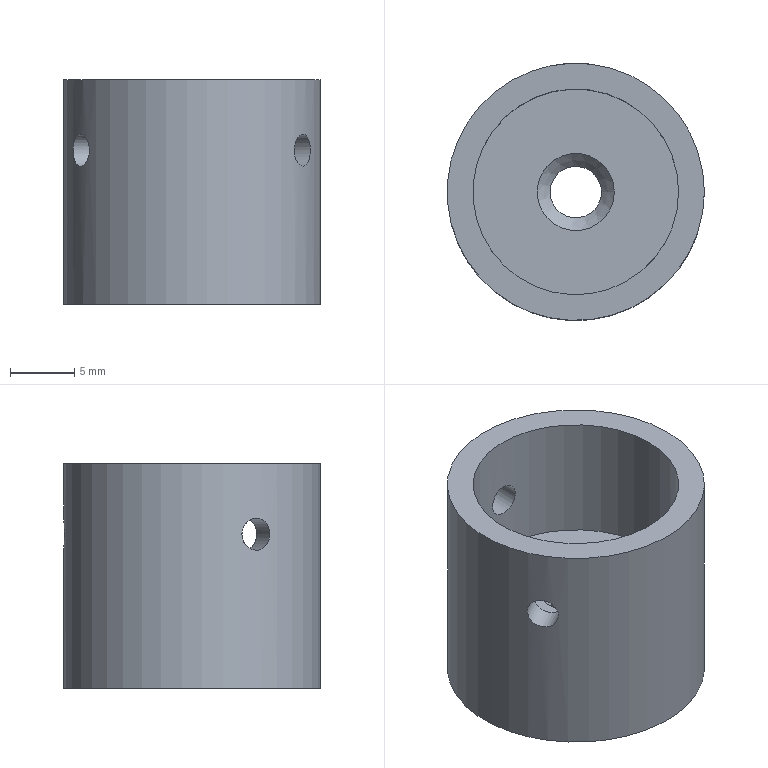Part | NX | features BREP 1, DATUM_CSYS 1 | 1 solid | 19 faces | box 20 x 20 x 17.5 mm | volume 3306 mm3 | cylinder 10 | plane 8 | cone 1 | commonest cylinder face diameters 6 x4 2.5 x3 4 x1 16 x1 20 x1
STEP:
#1=CARTESIAN_POINT('',(0.5952,-2.94,5.));
#2=VERTEX_POINT('',#1);
#3=CARTESIAN_POINT('',(2.94,-0.5952,5.));
#4=VERTEX_POINT('',#3);
#5=CARTESIAN_POINT('',(0.5952,-2.94,5.));
#6=DIRECTION('',(0.7071,0.7071,0.));
#7=VECTOR('',#6,1000.);
#8=LINE('',#5,#7);
#9=EDGE_CURVE('',#2,#4,#8,.T.);
#10=ORIENTED_EDGE('',*,*,#9,.F.);
#11=CARTESIAN_POINT('',(-0.5952,-2.94,5.));
#12=VERTEX_POINT('',#11);
#13=CARTESIAN_POINT('',(0.,0.,5.));
#14=DIRECTION('',(0.,0.,1.));
#15=DIRECTION('',(-0.1984,-0.9801,0.));
#16=AXIS2_PLACEMENT_3D('',#13,#14,#15);
#17=CIRCLE('',#16,3.);
#18=EDGE_CURVE('',#12,#2,#17,.T.);
#19=ORIENTED_EDGE('',*,*,#18,.F.);
#20=CARTESIAN_POINT('',(-2.94,-0.5952,5.));
#21=VERTEX_POINT('',#20);
#22=CARTESIAN_POINT('',(-2.94,-0.5952,5.));
#23=DIRECTION('',(0.7071,-0.7071,0.));
#24=VECTOR('',#23,1000.);
#25=LINE('',#22,#24);
#26=EDGE_CURVE('',#21,#12,#25,.T.);
#27=ORIENTED_EDGE('',*,*,#26,.F.);
#28=CARTESIAN_POINT('',(-2.94,0.5952,5.));
#29=VERTEX_POINT('',#28);
#30=CARTESIAN_POINT('',(0.,0.,5.));
#31=DIRECTION('',(0.,0.,1.));
#32=DIRECTION('',(-0.9801,0.1984,0.));
#33=AXIS2_PLACEMENT_3D('',#30,#31,#32);
#34=CIRCLE('',#33,3.);
#35=EDGE_CURVE('',#29,#21,#34,.T.);
#36=ORIENTED_EDGE('',*,*,#35,.F.);
#37=CARTESIAN_POINT('',(-0.5952,2.94,5.));
#38=VERTEX_POINT('',#37);
#39=CARTESIAN_POINT('',(-0.5952,2.94,5.));
#40=DIRECTION('',(-0.7071,-0.7071,0.));
#41=VECTOR('',#40,1000.);
#42=LINE('',#39,#41);
#43=EDGE_CURVE('',#38,#29,#42,.T.);
#44=ORIENTED_EDGE('',*,*,#43,.F.);
#45=CARTESIAN_POINT('',(0.5952,2.94,5.));
#46=VERTEX_POINT('',#45);
#47=CARTESIAN_POINT('',(0.,0.,5.));
#48=DIRECTION('',(0.,0.,1.));
#49=DIRECTION('',(0.1984,0.9801,0.));
#50=AXIS2_PLACEMENT_3D('',#47,#48,#49);
#51=CIRCLE('',#50,3.);
#52=EDGE_CURVE('',#46,#38,#51,.T.);
#53=ORIENTED_EDGE('',*,*,#52,.F.);
#54=CARTESIAN_POINT('',(2.94,0.5952,5.));
#55=VERTEX_POINT('',#54);
#56=CARTESIAN_POINT('',(2.94,0.5952,5.));
#57=DIRECTION('',(-0.7071,0.7071,0.));
#58=VECTOR('',#57,1000.);
#59=LINE('',#56,#58);
#60=EDGE_CURVE('',#55,#46,#59,.T.);
#61=ORIENTED_EDGE('',*,*,#60,.F.);
#62=CARTESIAN_POINT('',(0.,0.,5.));
#63=DIRECTION('',(0.,0.,1.));
#64=DIRECTION('',(0.9801,-0.1984,0.));
#65=AXIS2_PLACEMENT_3D('',#62,#63,#64);
#66=CIRCLE('',#65,3.);
#67=EDGE_CURVE('',#4,#55,#66,.T.);
#68=ORIENTED_EDGE('',*,*,#67,.F.);
#69=EDGE_LOOP('',(#10,#19,#27,#36,#44,#53,#61,#68));
#70=FACE_BOUND('',#69,.T.);
#71=CARTESIAN_POINT('',(2.,0.,5.));
#72=VERTEX_POINT('',#71);
#73=CARTESIAN_POINT('',(0.,0.,5.));
#74=DIRECTION('',(0.,0.,-1.));
#75=DIRECTION('',(1.,0.,0.));
#76=AXIS2_PLACEMENT_3D('',#73,#74,#75);
#77=CIRCLE('',#76,2.);
#78=EDGE_CURVE('',#72,#72,#77,.T.);
#79=ORIENTED_EDGE('',*,*,#78,.F.);
#80=EDGE_LOOP('',(#79));
#81=FACE_BOUND('',#80,.T.);
#82=CARTESIAN_POINT('',(0.,0.,5.));
#83=DIRECTION('',(0.,0.,1.));
#84=DIRECTION('',(1.,0.,0.));
#85=AXIS2_PLACEMENT_3D('',#82,#83,#84);
#86=PLANE('',#85);
#87=ADVANCED_FACE('',(#70,#81),#86,.F.);
#88=ORIENTED_EDGE('',*,*,#67,.T.);
#89=CARTESIAN_POINT('',(2.94,0.5952,0.5));
#90=VERTEX_POINT('',#89);
#91=CARTESIAN_POINT('',(2.94,0.5952,5.));
#92=DIRECTION('',(0.,0.,-1.));
#93=VECTOR('',#92,1000.);
#94=LINE('',#91,#93);
#95=EDGE_CURVE('',#55,#90,#94,.T.);
#96=ORIENTED_EDGE('',*,*,#95,.T.);
#97=CARTESIAN_POINT('',(2.94,-0.5952,0.5));
#98=VERTEX_POINT('',#97);
#99=CARTESIAN_POINT('',(0.,0.,0.5));
#100=DIRECTION('',(0.,0.,-1.));
#101=DIRECTION('',(0.9801,0.1984,0.));
#102=AXIS2_PLACEMENT_3D('',#99,#100,#101);
#103=CIRCLE('',#102,3.);
#104=EDGE_CURVE('',#90,#98,#103,.T.);
#105=ORIENTED_EDGE('',*,*,#104,.T.);
#106=CARTESIAN_POINT('',(2.94,-0.5952,5.));
#107=DIRECTION('',(0.,0.,-1.));
#108=VECTOR('',#107,1000.);
#109=LINE('',#106,#108);
#110=EDGE_CURVE('',#4,#98,#109,.T.);
#111=ORIENTED_EDGE('',*,*,#110,.F.);
#112=EDGE_LOOP('',(#88,#96,#105,#111));
#113=FACE_BOUND('',#112,.T.);
#114=CARTESIAN_POINT('',(0.,0.,5.));
#115=DIRECTION('',(0.,0.,-1.));
#116=DIRECTION('',(-0.9801,0.1984,0.));
#117=AXIS2_PLACEMENT_3D('',#114,#115,#116);
#118=CYLINDRICAL_SURFACE('',#117,3.);
#119=ADVANCED_FACE('',(#113),#118,.F.);
#120=ORIENTED_EDGE('',*,*,#60,.T.);
#121=CARTESIAN_POINT('',(0.5952,2.94,0.5));
#122=VERTEX_POINT('',#121);
#123=CARTESIAN_POINT('',(0.5952,2.94,5.));
#124=DIRECTION('',(0.,0.,-1.));
#125=VECTOR('',#124,1000.);
#126=LINE('',#123,#125);
#127=EDGE_CURVE('',#46,#122,#126,.T.);
#128=ORIENTED_EDGE('',*,*,#127,.T.);
#129=CARTESIAN_POINT('',(0.5952,2.94,0.5));
#130=DIRECTION('',(0.7071,-0.7071,0.));
#131=VECTOR('',#130,1000.);
#132=LINE('',#129,#131);
#133=EDGE_CURVE('',#122,#90,#132,.T.);
#134=ORIENTED_EDGE('',*,*,#133,.T.);
#135=ORIENTED_EDGE('',*,*,#95,.F.);
#136=EDGE_LOOP('',(#120,#128,#134,#135));
#137=FACE_BOUND('',#136,.T.);
#138=CARTESIAN_POINT('',(1.768,1.768,1.85));
#139=DIRECTION('',(-0.7071,-0.7071,0.));
#140=DIRECTION('',(0.7071,-0.7071,0.));
#141=AXIS2_PLACEMENT_3D('',#138,#139,#140);
#142=PLANE('',#141);
#143=ADVANCED_FACE('',(#137),#142,.T.);
#144=ORIENTED_EDGE('',*,*,#52,.T.);
#145=CARTESIAN_POINT('',(-0.5952,2.94,0.5));
#146=VERTEX_POINT('',#145);
#147=CARTESIAN_POINT('',(-0.5952,2.94,5.));
#148=DIRECTION('',(0.,0.,-1.));
#149=VECTOR('',#148,1000.);
#150=LINE('',#147,#149);
#151=EDGE_CURVE('',#38,#146,#150,.T.);
#152=ORIENTED_EDGE('',*,*,#151,.T.);
#153=CARTESIAN_POINT('',(0.,0.,0.5));
#154=DIRECTION('',(0.,0.,-1.));
#155=DIRECTION('',(-0.1984,0.9801,0.));
#156=AXIS2_PLACEMENT_3D('',#153,#154,#155);
#157=CIRCLE('',#156,3.);
#158=EDGE_CURVE('',#146,#122,#157,.T.);
#159=ORIENTED_EDGE('',*,*,#158,.T.);
#160=ORIENTED_EDGE('',*,*,#127,.F.);
#161=EDGE_LOOP('',(#144,#152,#159,#160));
#162=FACE_BOUND('',#161,.T.);
#163=CARTESIAN_POINT('',(0.,0.,5.));
#164=DIRECTION('',(0.,0.,-1.));
#165=DIRECTION('',(-0.1984,-0.9801,0.));
#166=AXIS2_PLACEMENT_3D('',#163,#164,#165);
#167=CYLINDRICAL_SURFACE('',#166,3.);
#168=ADVANCED_FACE('',(#162),#167,.F.);
#169=ORIENTED_EDGE('',*,*,#43,.T.);
#170=CARTESIAN_POINT('',(-2.94,0.5952,0.5));
#171=VERTEX_POINT('',#170);
#172=CARTESIAN_POINT('',(-2.94,0.5952,5.));
#173=DIRECTION('',(0.,0.,-1.));
#174=VECTOR('',#173,1000.);
#175=LINE('',#172,#174);
#176=EDGE_CURVE('',#29,#171,#175,.T.);
#177=ORIENTED_EDGE('',*,*,#176,.T.);
#178=CARTESIAN_POINT('',(-2.94,0.5952,0.5));
#179=DIRECTION('',(0.7071,0.7071,0.));
#180=VECTOR('',#179,1000.);
#181=LINE('',#178,#180);
#182=EDGE_CURVE('',#171,#146,#181,.T.);
#183=ORIENTED_EDGE('',*,*,#182,.T.);
#184=ORIENTED_EDGE('',*,*,#151,.F.);
#185=EDGE_LOOP('',(#169,#177,#183,#184));
#186=FACE_BOUND('',#185,.T.);
#187=CARTESIAN_POINT('',(-1.768,1.768,1.85));
#188=DIRECTION('',(0.7071,-0.7071,0.));
#189=DIRECTION('',(0.7071,0.7071,0.));
#190=AXIS2_PLACEMENT_3D('',#187,#188,#189);
#191=PLANE('',#190);
#192=ADVANCED_FACE('',(#186),#191,.T.);
#193=ORIENTED_EDGE('',*,*,#35,.T.);
#194=CARTESIAN_POINT('',(-2.94,-0.5952,0.5));
#195=VERTEX_POINT('',#194);
#196=CARTESIAN_POINT('',(-2.94,-0.5952,5.));
#197=DIRECTION('',(0.,0.,-1.));
#198=VECTOR('',#197,1000.);
#199=LINE('',#196,#198);
#200=EDGE_CURVE('',#21,#195,#199,.T.);
#201=ORIENTED_EDGE('',*,*,#200,.T.);
#202=CARTESIAN_POINT('',(0.,0.,0.5));
#203=DIRECTION('',(0.,0.,-1.));
#204=DIRECTION('',(-0.9801,-0.1984,0.));
#205=AXIS2_PLACEMENT_3D('',#202,#203,#204);
#206=CIRCLE('',#205,3.);
#207=EDGE_CURVE('',#195,#171,#206,.T.);
#208=ORIENTED_EDGE('',*,*,#207,.T.);
#209=ORIENTED_EDGE('',*,*,#176,.F.);
#210=EDGE_LOOP('',(#193,#201,#208,#209));
#211=FACE_BOUND('',#210,.T.);
#212=CARTESIAN_POINT('',(0.,0.,5.));
#213=DIRECTION('',(0.,0.,-1.));
#214=DIRECTION('',(0.9801,-0.1984,0.));
#215=AXIS2_PLACEMENT_3D('',#212,#213,#214);
#216=CYLINDRICAL_SURFACE('',#215,3.);
#217=ADVANCED_FACE('',(#211),#216,.F.);
#218=ORIENTED_EDGE('',*,*,#26,.T.);
#219=CARTESIAN_POINT('',(-0.5952,-2.94,0.5));
#220=VERTEX_POINT('',#219);
#221=CARTESIAN_POINT('',(-0.5952,-2.94,5.));
#222=DIRECTION('',(0.,0.,-1.));
#223=VECTOR('',#222,1000.);
#224=LINE('',#221,#223);
#225=EDGE_CURVE('',#12,#220,#224,.T.);
#226=ORIENTED_EDGE('',*,*,#225,.T.);
#227=CARTESIAN_POINT('',(-0.5952,-2.94,0.5));
#228=DIRECTION('',(-0.7071,0.7071,0.));
#229=VECTOR('',#228,1000.);
#230=LINE('',#227,#229);
#231=EDGE_CURVE('',#220,#195,#230,.T.);
#232=ORIENTED_EDGE('',*,*,#231,.T.);
#233=ORIENTED_EDGE('',*,*,#200,.F.);
#234=EDGE_LOOP('',(#218,#226,#232,#233));
#235=FACE_BOUND('',#234,.T.);
#236=CARTESIAN_POINT('',(-1.768,-1.768,1.85));
#237=DIRECTION('',(0.7071,0.7071,0.));
#238=DIRECTION('',(-0.7071,0.7071,0.));
#239=AXIS2_PLACEMENT_3D('',#236,#237,#238);
#240=PLANE('',#239);
#241=ADVANCED_FACE('',(#235),#240,.T.);
#242=ORIENTED_EDGE('',*,*,#18,.T.);
#243=CARTESIAN_POINT('',(0.5952,-2.94,0.5));
#244=VERTEX_POINT('',#243);
#245=CARTESIAN_POINT('',(0.5952,-2.94,5.));
#246=DIRECTION('',(0.,0.,-1.));
#247=VECTOR('',#246,1000.);
#248=LINE('',#245,#247);
#249=EDGE_CURVE('',#2,#244,#248,.T.);
#250=ORIENTED_EDGE('',*,*,#249,.T.);
#251=CARTESIAN_POINT('',(0.,0.,0.5));
#252=DIRECTION('',(0.,0.,-1.));
#253=DIRECTION('',(0.1984,-0.9801,0.));
#254=AXIS2_PLACEMENT_3D('',#251,#252,#253);
#255=CIRCLE('',#254,3.);
#256=EDGE_CURVE('',#244,#220,#255,.T.);
#257=ORIENTED_EDGE('',*,*,#256,.T.);
#258=ORIENTED_EDGE('',*,*,#225,.F.);
#259=EDGE_LOOP('',(#242,#250,#257,#258));
#260=FACE_BOUND('',#259,.T.);
#261=CARTESIAN_POINT('',(0.,0.,5.));
#262=DIRECTION('',(0.,0.,-1.));
#263=DIRECTION('',(0.1984,0.9801,0.));
#264=AXIS2_PLACEMENT_3D('',#261,#262,#263);
#265=CYLINDRICAL_SURFACE('',#264,3.);
#266=ADVANCED_FACE('',(#260),#265,.F.);
#267=ORIENTED_EDGE('',*,*,#9,.T.);
#268=ORIENTED_EDGE('',*,*,#110,.T.);
#269=CARTESIAN_POINT('',(2.94,-0.5952,0.5));
#270=DIRECTION('',(-0.7071,-0.7071,0.));
#271=VECTOR('',#270,1000.);
#272=LINE('',#269,#271);
#273=EDGE_CURVE('',#98,#244,#272,.T.);
#274=ORIENTED_EDGE('',*,*,#273,.T.);
#275=ORIENTED_EDGE('',*,*,#249,.F.);
#276=EDGE_LOOP('',(#267,#268,#274,#275));
#277=FACE_BOUND('',#276,.T.);
#278=CARTESIAN_POINT('',(1.768,-1.768,1.85));
#279=DIRECTION('',(-0.7071,0.7071,0.));
#280=DIRECTION('',(-0.7071,-0.7071,0.));
#281=AXIS2_PLACEMENT_3D('',#278,#279,#280);
#282=PLANE('',#281);
#283=ADVANCED_FACE('',(#277),#282,.T.);
#284=CARTESIAN_POINT('',(10.,0.,0.5));
#285=VERTEX_POINT('',#284);
#286=CARTESIAN_POINT('',(0.,0.,0.5));
#287=DIRECTION('',(0.,0.,1.));
#288=DIRECTION('',(1.,0.,0.));
#289=AXIS2_PLACEMENT_3D('',#286,#287,#288);
#290=CIRCLE('',#289,10.);
#291=EDGE_CURVE('',#285,#285,#290,.T.);
#292=ORIENTED_EDGE('',*,*,#291,.F.);
#293=EDGE_LOOP('',(#292));
#294=FACE_BOUND('',#293,.T.);
#295=ORIENTED_EDGE('',*,*,#182,.F.);
#296=ORIENTED_EDGE('',*,*,#207,.F.);
#297=ORIENTED_EDGE('',*,*,#231,.F.);
#298=ORIENTED_EDGE('',*,*,#256,.F.);
#299=ORIENTED_EDGE('',*,*,#273,.F.);
#300=ORIENTED_EDGE('',*,*,#104,.F.);
#301=ORIENTED_EDGE('',*,*,#133,.F.);
#302=ORIENTED_EDGE('',*,*,#158,.F.);
#303=EDGE_LOOP('',(#295,#296,#297,#298,#299,#300,#301,#302));
#304=FACE_BOUND('',#303,.T.);
#305=CARTESIAN_POINT('',(0.,0.,0.5));
#306=DIRECTION('',(0.,0.,1.));
#307=DIRECTION('',(-1.,0.,0.));
#308=AXIS2_PLACEMENT_3D('',#305,#306,#307);
#309=PLANE('',#308);
#310=ADVANCED_FACE('',(#294,#304),#309,.F.);
#311=ORIENTED_EDGE('',*,*,#291,.T.);
#312=CARTESIAN_POINT('',(10.,0.,18.));
#313=VERTEX_POINT('',#312);
#314=CARTESIAN_POINT('',(10.,0.,0.5));
#315=DIRECTION('',(0.,0.,1.));
#316=VECTOR('',#315,1000.);
#317=LINE('',#314,#316);
#318=EDGE_CURVE('',#285,#313,#317,.T.);
#319=ORIENTED_EDGE('',*,*,#318,.T.);
#320=CARTESIAN_POINT('',(0.,0.,18.));
#321=DIRECTION('',(0.,0.,1.));
#322=DIRECTION('',(1.,0.,0.));
#323=AXIS2_PLACEMENT_3D('',#320,#321,#322);
#324=CIRCLE('',#323,10.);
#325=EDGE_CURVE('',#313,#313,#324,.T.);
#326=ORIENTED_EDGE('',*,*,#325,.F.);
#327=ORIENTED_EDGE('',*,*,#318,.F.);
#328=EDGE_LOOP('',(#311,#319,#326,#327));
#329=FACE_BOUND('',#328,.T.);
#330=CARTESIAN_POINT('',(-9.217,-3.878,12.5));
#331=VERTEX_POINT('',#330);
#332=CARTESIAN_POINT('',(-9.116,-4.133,13.481));
#333=CARTESIAN_POINT('',(-9.268,-3.751,12.5));
#334=CARTESIAN_POINT('',(-9.116,-4.133,11.52));
#335=CARTESIAN_POINT('',(-8.678,-5.009,11.115));
#336=CARTESIAN_POINT('',(-8.137,-5.829,11.52));
#337=CARTESIAN_POINT('',(-7.883,-6.15,12.5));
#338=CARTESIAN_POINT('',(-8.136,-5.83,13.478));
#339=CARTESIAN_POINT('',(-8.677,-5.011,13.885));
#340=CARTESIAN_POINT('',(-9.116,-4.133,13.481));
#341=CARTESIAN_POINT('',(-9.268,-3.751,12.5));
#342=CARTESIAN_POINT('',(-9.116,-4.133,11.52));
#343=B_SPLINE_CURVE_WITH_KNOTS('',3,(#332,#333,#334,#335,#336,#337,#338,#339,#340,#341,#342),.UNSPECIFIED.,.T.,.F.,(1,1,1,1,1,1,1,1,1,1,1,1,1,1,1),(-0.002934,-0.001956,-0.0009779,0.,0.0009779,0.001956,0.002934,0.003911,0.004889,0.005867,0.006845,0.007823,0.008801,0.009779,0.01076),.UNSPECIFIED.);
#344=EDGE_CURVE('',#331,#331,#343,.T.);
#345=ORIENTED_EDGE('',*,*,#344,.F.);
#346=EDGE_LOOP('',(#345));
#347=FACE_BOUND('',#346,.T.);
#348=CARTESIAN_POINT('',(1.25,9.922,12.5));
#349=VERTEX_POINT('',#348);
#350=CARTESIAN_POINT('',(0.9787,9.961,13.481));
#351=CARTESIAN_POINT('',(1.386,9.902,12.5));
#352=CARTESIAN_POINT('',(0.979,9.961,11.52));
#353=CARTESIAN_POINT('',(0.001122,10.02,11.115));
#354=CARTESIAN_POINT('',(-0.9793,9.961,11.52));
#355=CARTESIAN_POINT('',(-1.385,9.902,12.5));
#356=CARTESIAN_POINT('',(-0.9805,9.961,13.478));
#357=CARTESIAN_POINT('',(-0.001244,10.02,13.885));
#358=CARTESIAN_POINT('',(0.9787,9.961,13.481));
#359=CARTESIAN_POINT('',(1.386,9.902,12.5));
#360=CARTESIAN_POINT('',(0.979,9.961,11.52));
#361=B_SPLINE_CURVE_WITH_KNOTS('',3,(#350,#351,#352,#353,#354,#355,#356,#357,#358,#359,#360),.UNSPECIFIED.,.T.,.F.,(1,1,1,1,1,1,1,1,1,1,1,1,1,1,1),(-0.002934,-0.001956,-0.0009779,0.,0.0009779,0.001956,0.002934,0.003911,0.004889,0.005867,0.006845,0.007823,0.008801,0.009779,0.01076),.UNSPECIFIED.);
#362=EDGE_CURVE('',#349,#349,#361,.T.);
#363=ORIENTED_EDGE('',*,*,#362,.F.);
#364=EDGE_LOOP('',(#363));
#365=FACE_BOUND('',#364,.T.);
#366=CARTESIAN_POINT('',(7.967,-6.043,12.5));
#367=VERTEX_POINT('',#366);
#368=CARTESIAN_POINT('',(8.137,-5.828,13.481));
#369=CARTESIAN_POINT('',(7.882,-6.151,12.5));
#370=CARTESIAN_POINT('',(8.137,-5.828,11.52));
#371=CARTESIAN_POINT('',(8.677,-5.011,11.115));
#372=CARTESIAN_POINT('',(9.116,-4.132,11.52));
#373=CARTESIAN_POINT('',(9.268,-3.751,12.5));
#374=CARTESIAN_POINT('',(9.117,-4.131,13.478));
#375=CARTESIAN_POINT('',(8.678,-5.009,13.885));
#376=CARTESIAN_POINT('',(8.137,-5.828,13.481));
#377=CARTESIAN_POINT('',(7.882,-6.151,12.5));
#378=CARTESIAN_POINT('',(8.137,-5.828,11.52));
#379=B_SPLINE_CURVE_WITH_KNOTS('',3,(#368,#369,#370,#371,#372,#373,#374,#375,#376,#377,#378),.UNSPECIFIED.,.T.,.F.,(1,1,1,1,1,1,1,1,1,1,1,1,1,1,1),(-0.002934,-0.001956,-0.0009779,0.,0.0009779,0.001956,0.002934,0.003911,0.004889,0.005867,0.006845,0.007823,0.008801,0.009779,0.01076),.UNSPECIFIED.);
#380=EDGE_CURVE('',#367,#367,#379,.T.);
#381=ORIENTED_EDGE('',*,*,#380,.F.);
#382=EDGE_LOOP('',(#381));
#383=FACE_BOUND('',#382,.T.);
#384=CARTESIAN_POINT('',(0.,0.,0.));
#385=DIRECTION('',(0.,0.,1.));
#386=DIRECTION('',(-1.,0.,0.));
#387=AXIS2_PLACEMENT_3D('',#384,#385,#386);
#388=CYLINDRICAL_SURFACE('',#387,10.);
#389=ADVANCED_FACE('',(#329,#347,#365,#383),#388,.T.);
#390=ORIENTED_EDGE('',*,*,#325,.T.);
#391=EDGE_LOOP('',(#390));
#392=FACE_BOUND('',#391,.T.);
#393=CARTESIAN_POINT('',(8.,0.,18.));
#394=VERTEX_POINT('',#393);
#395=CARTESIAN_POINT('',(0.,0.,18.));
#396=DIRECTION('',(0.,0.,-1.));
#397=DIRECTION('',(1.,0.,0.));
#398=AXIS2_PLACEMENT_3D('',#395,#396,#397);
#399=CIRCLE('',#398,8.);
#400=EDGE_CURVE('',#394,#394,#399,.T.);
#401=ORIENTED_EDGE('',*,*,#400,.T.);
#402=EDGE_LOOP('',(#401));
#403=FACE_BOUND('',#402,.T.);
#404=CARTESIAN_POINT('',(0.,0.,18.));
#405=DIRECTION('',(0.,0.,1.));
#406=DIRECTION('',(-1.,0.,0.));
#407=AXIS2_PLACEMENT_3D('',#404,#405,#406);
#408=PLANE('',#407);
#409=ADVANCED_FACE('',(#392,#403),#408,.T.);
#410=CARTESIAN_POINT('',(8.,0.,8.));
#411=VERTEX_POINT('',#410);
#412=CARTESIAN_POINT('',(8.,0.,18.));
#413=DIRECTION('',(0.,0.,-1.));
#414=VECTOR('',#413,1000.);
#415=LINE('',#412,#414);
#416=EDGE_CURVE('',#394,#411,#415,.T.);
#417=ORIENTED_EDGE('',*,*,#416,.T.);
#418=CARTESIAN_POINT('',(0.,0.,8.));
#419=DIRECTION('',(0.,0.,-1.));
#420=DIRECTION('',(1.,0.,0.));
#421=AXIS2_PLACEMENT_3D('',#418,#419,#420);
#422=CIRCLE('',#421,8.);
#423=EDGE_CURVE('',#411,#411,#422,.T.);
#424=ORIENTED_EDGE('',*,*,#423,.T.);
#425=ORIENTED_EDGE('',*,*,#416,.F.);
#426=ORIENTED_EDGE('',*,*,#400,.F.);
#427=EDGE_LOOP('',(#417,#424,#425,#426));
#428=FACE_BOUND('',#427,.T.);
#429=CARTESIAN_POINT('',(-7.468,-2.868,12.5));
#430=VERTEX_POINT('',#429);
#431=CARTESIAN_POINT('',(-7.375,-3.128,11.519));
#432=CARTESIAN_POINT('',(-7.514,-2.739,12.5));
#433=CARTESIAN_POINT('',(-7.375,-3.128,13.48));
#434=CARTESIAN_POINT('',(-6.95,-4.011,13.885));
#435=CARTESIAN_POINT('',(-6.396,-4.824,13.48));
#436=CARTESIAN_POINT('',(-6.129,-5.138,12.5));
#437=CARTESIAN_POINT('',(-6.396,-4.825,11.522));
#438=CARTESIAN_POINT('',(-6.949,-4.013,11.115));
#439=CARTESIAN_POINT('',(-7.375,-3.128,11.519));
#440=CARTESIAN_POINT('',(-7.514,-2.739,12.5));
#441=CARTESIAN_POINT('',(-7.375,-3.128,13.48));
#442=B_SPLINE_CURVE_WITH_KNOTS('',3,(#431,#432,#433,#434,#435,#436,#437,#438,#439,#440,#441),.UNSPECIFIED.,.T.,.F.,(1,1,1,1,1,1,1,1,1,1,1,1,1,1,1),(-0.002935,-0.001957,-0.0009784,0.,0.0009784,0.001957,0.002935,0.003914,0.004892,0.00587,0.006849,0.007827,0.008806,0.009784,0.01076),.UNSPECIFIED.);
#443=EDGE_CURVE('',#430,#430,#442,.T.);
#444=ORIENTED_EDGE('',*,*,#443,.F.);
#445=EDGE_LOOP('',(#444));
#446=FACE_BOUND('',#445,.T.);
#447=CARTESIAN_POINT('',(1.25,7.902,12.5));
#448=VERTEX_POINT('',#447);
#449=CARTESIAN_POINT('',(0.9787,7.951,11.519));
#450=CARTESIAN_POINT('',(1.386,7.877,12.5));
#451=CARTESIAN_POINT('',(0.979,7.951,13.48));
#452=CARTESIAN_POINT('',(0.001184,8.024,13.885));
#453=CARTESIAN_POINT('',(-0.9795,7.951,13.48));
#454=CARTESIAN_POINT('',(-1.385,7.877,12.5));
#455=CARTESIAN_POINT('',(-0.9805,7.951,11.522));
#456=CARTESIAN_POINT('',(-0.001093,8.024,11.115));
#457=CARTESIAN_POINT('',(0.9787,7.951,11.519));
#458=CARTESIAN_POINT('',(1.386,7.877,12.5));
#459=CARTESIAN_POINT('',(0.979,7.951,13.48));
#460=B_SPLINE_CURVE_WITH_KNOTS('',3,(#449,#450,#451,#452,#453,#454,#455,#456,#457,#458,#459),.UNSPECIFIED.,.T.,.F.,(1,1,1,1,1,1,1,1,1,1,1,1,1,1,1),(-0.002935,-0.001957,-0.0009784,0.,0.0009784,0.001957,0.002935,0.003914,0.004892,0.00587,0.006849,0.007827,0.008806,0.009784,0.01076),.UNSPECIFIED.);
#461=EDGE_CURVE('',#448,#448,#460,.T.);
#462=ORIENTED_EDGE('',*,*,#461,.F.);
#463=EDGE_LOOP('',(#462));
#464=FACE_BOUND('',#463,.T.);
#465=CARTESIAN_POINT('',(6.218,-5.033,12.5));
#466=VERTEX_POINT('',#465);
#467=CARTESIAN_POINT('',(6.397,-4.823,11.519));
#468=CARTESIAN_POINT('',(6.129,-5.138,12.5));
#469=CARTESIAN_POINT('',(6.396,-4.823,13.48));
#470=CARTESIAN_POINT('',(6.949,-4.013,13.885));
#471=CARTESIAN_POINT('',(7.376,-3.127,13.48));
#472=CARTESIAN_POINT('',(7.514,-2.739,12.5));
#473=CARTESIAN_POINT('',(7.376,-3.126,11.522));
#474=CARTESIAN_POINT('',(6.95,-4.011,11.115));
#475=CARTESIAN_POINT('',(6.397,-4.823,11.519));
#476=CARTESIAN_POINT('',(6.129,-5.138,12.5));
#477=CARTESIAN_POINT('',(6.396,-4.823,13.48));
#478=B_SPLINE_CURVE_WITH_KNOTS('',3,(#467,#468,#469,#470,#471,#472,#473,#474,#475,#476,#477),.UNSPECIFIED.,.T.,.F.,(1,1,1,1,1,1,1,1,1,1,1,1,1,1,1),(-0.002935,-0.001957,-0.0009784,0.,0.0009784,0.001957,0.002935,0.003914,0.004892,0.00587,0.006849,0.007827,0.008806,0.009784,0.01076),.UNSPECIFIED.);
#479=EDGE_CURVE('',#466,#466,#478,.T.);
#480=ORIENTED_EDGE('',*,*,#479,.F.);
#481=EDGE_LOOP('',(#480));
#482=FACE_BOUND('',#481,.T.);
#483=CARTESIAN_POINT('',(0.,0.,18.));
#484=DIRECTION('',(0.,0.,-1.));
#485=DIRECTION('',(-1.,0.,0.));
#486=AXIS2_PLACEMENT_3D('',#483,#484,#485);
#487=CYLINDRICAL_SURFACE('',#486,8.);
#488=ADVANCED_FACE('',(#428,#446,#464,#482),#487,.F.);
#489=ORIENTED_EDGE('',*,*,#423,.F.);
#490=EDGE_LOOP('',(#489));
#491=FACE_BOUND('',#490,.T.);
#492=CARTESIAN_POINT('',(3.,0.,8.));
#493=VERTEX_POINT('',#492);
#494=CARTESIAN_POINT('',(0.,0.,8.));
#495=DIRECTION('',(0.,0.,-1.));
#496=DIRECTION('',(1.,0.,0.));
#497=AXIS2_PLACEMENT_3D('',#494,#495,#496);
#498=CIRCLE('',#497,3.);
#499=EDGE_CURVE('',#493,#493,#498,.T.);
#500=ORIENTED_EDGE('',*,*,#499,.T.);
#501=EDGE_LOOP('',(#500));
#502=FACE_BOUND('',#501,.T.);
#503=CARTESIAN_POINT('',(0.,0.,8.));
#504=DIRECTION('',(0.,0.,-1.));
#505=DIRECTION('',(-1.,0.,0.));
#506=AXIS2_PLACEMENT_3D('',#503,#504,#505);
#507=PLANE('',#506);
#508=ADVANCED_FACE('',(#491,#502),#507,.F.);
#509=CARTESIAN_POINT('',(1.25,7.902,12.5));
#510=DIRECTION('',(0.,1.,0.));
#511=VECTOR('',#510,1000.);
#512=LINE('',#509,#511);
#513=EDGE_CURVE('',#448,#349,#512,.T.);
#514=ORIENTED_EDGE('',*,*,#513,.T.);
#515=ORIENTED_EDGE('',*,*,#362,.T.);
#516=ORIENTED_EDGE('',*,*,#513,.F.);
#517=ORIENTED_EDGE('',*,*,#461,.T.);
#518=EDGE_LOOP('',(#514,#515,#516,#517));
#519=FACE_BOUND('',#518,.T.);
#520=CARTESIAN_POINT('',(0.,7.8,12.5));
#521=DIRECTION('',(0.,1.,0.));
#522=DIRECTION('',(-1.,0.,0.));
#523=AXIS2_PLACEMENT_3D('',#520,#521,#522);
#524=CYLINDRICAL_SURFACE('',#523,1.25);
#525=ADVANCED_FACE('',(#519),#524,.F.);
#526=CARTESIAN_POINT('',(-7.468,-2.868,12.5));
#527=DIRECTION('',(-0.866,-0.5,0.));
#528=VECTOR('',#527,1000.);
#529=LINE('',#526,#528);
#530=EDGE_CURVE('',#430,#331,#529,.T.);
#531=ORIENTED_EDGE('',*,*,#530,.T.);
#532=ORIENTED_EDGE('',*,*,#344,.T.);
#533=ORIENTED_EDGE('',*,*,#530,.F.);
#534=ORIENTED_EDGE('',*,*,#443,.T.);
#535=EDGE_LOOP('',(#531,#532,#533,#534));
#536=FACE_BOUND('',#535,.T.);
#537=CARTESIAN_POINT('',(-6.755,-3.9,12.5));
#538=DIRECTION('',(-0.866,-0.5,0.));
#539=DIRECTION('',(0.5,-0.866,0.));
#540=AXIS2_PLACEMENT_3D('',#537,#538,#539);
#541=CYLINDRICAL_SURFACE('',#540,1.25);
#542=ADVANCED_FACE('',(#536),#541,.F.);
#543=CARTESIAN_POINT('',(6.218,-5.033,12.5));
#544=DIRECTION('',(0.866,-0.5,0.));
#545=VECTOR('',#544,1000.);
#546=LINE('',#543,#545);
#547=EDGE_CURVE('',#466,#367,#546,.T.);
#548=ORIENTED_EDGE('',*,*,#547,.T.);
#549=ORIENTED_EDGE('',*,*,#380,.T.);
#550=ORIENTED_EDGE('',*,*,#547,.F.);
#551=ORIENTED_EDGE('',*,*,#479,.T.);
#552=EDGE_LOOP('',(#548,#549,#550,#551));
#553=FACE_BOUND('',#552,.T.);
#554=CARTESIAN_POINT('',(6.755,-3.9,12.5));
#555=DIRECTION('',(0.866,-0.5,0.));
#556=DIRECTION('',(0.5,0.866,0.));
#557=AXIS2_PLACEMENT_3D('',#554,#555,#556);
#558=CYLINDRICAL_SURFACE('',#557,1.25);
#559=ADVANCED_FACE('',(#553),#558,.F.);
#560=CARTESIAN_POINT('',(2.,0.,7.));
#561=VERTEX_POINT('',#560);
#562=CARTESIAN_POINT('',(2.,0.,7.));
#563=DIRECTION('',(0.,0.,-1.));
#564=VECTOR('',#563,1000.);
#565=LINE('',#562,#564);
#566=EDGE_CURVE('',#561,#72,#565,.T.);
#567=ORIENTED_EDGE('',*,*,#566,.T.);
#568=ORIENTED_EDGE('',*,*,#78,.T.);
#569=ORIENTED_EDGE('',*,*,#566,.F.);
#570=CARTESIAN_POINT('',(0.,0.,7.));
#571=DIRECTION('',(0.,0.,-1.));
#572=DIRECTION('',(1.,0.,0.));
#573=AXIS2_PLACEMENT_3D('',#570,#571,#572);
#574=CIRCLE('',#573,2.);
#575=EDGE_CURVE('',#561,#561,#574,.T.);
#576=ORIENTED_EDGE('',*,*,#575,.F.);
#577=EDGE_LOOP('',(#567,#568,#569,#576));
#578=FACE_BOUND('',#577,.T.);
#579=CARTESIAN_POINT('',(0.,0.,7.));
#580=DIRECTION('',(0.,0.,-1.));
#581=DIRECTION('',(-1.,0.,0.));
#582=AXIS2_PLACEMENT_3D('',#579,#580,#581);
#583=CYLINDRICAL_SURFACE('',#582,2.);
#584=ADVANCED_FACE('',(#578),#583,.F.);
#585=CARTESIAN_POINT('',(3.,0.,8.));
#586=DIRECTION('',(-0.7071,0.,-0.7071));
#587=VECTOR('',#586,1000.);
#588=LINE('',#585,#587);
#589=EDGE_CURVE('',#493,#561,#588,.T.);
#590=ORIENTED_EDGE('',*,*,#589,.T.);
#591=ORIENTED_EDGE('',*,*,#575,.T.);
#592=ORIENTED_EDGE('',*,*,#589,.F.);
#593=ORIENTED_EDGE('',*,*,#499,.F.);
#594=EDGE_LOOP('',(#590,#591,#592,#593));
#595=FACE_BOUND('',#594,.T.);
#596=CARTESIAN_POINT('',(0.,0.,7.));
#597=DIRECTION('',(0.,0.,1.));
#598=DIRECTION('',(-1.,0.,0.));
#599=AXIS2_PLACEMENT_3D('',#596,#597,#598);
#600=CONICAL_SURFACE('',#599,2.,0.7854);
#601=ADVANCED_FACE('',(#595),#600,.F.);
#602=CLOSED_SHELL('',(#87,#119,#143,#168,#192,#217,#241,#266,#283,#310,#389,#409,#488,#508,#525,#542,#559,#584,#601));
#603=MANIFOLD_SOLID_BREP('',#602);
#604=(LENGTH_UNIT()NAMED_UNIT(*)SI_UNIT(.MILLI.,.METRE.));
#605=UNCERTAINTY_MEASURE_WITH_UNIT(LENGTH_MEASURE(0.0508),#604,'','');
#606=(NAMED_UNIT(*)PLANE_ANGLE_UNIT()SI_UNIT($,.RADIAN.));
#607=(NAMED_UNIT(*)SI_UNIT($,.STERADIAN.)SOLID_ANGLE_UNIT());
#608=(GEOMETRIC_REPRESENTATION_CONTEXT(3)GLOBAL_UNCERTAINTY_ASSIGNED_CONTEXT((#605))GLOBAL_UNIT_ASSIGNED_CONTEXT((#604,#606,#607))REPRESENTATION_CONTEXT('',''));
#609=ADVANCED_BREP_SHAPE_REPRESENTATION('',(#603),#608);